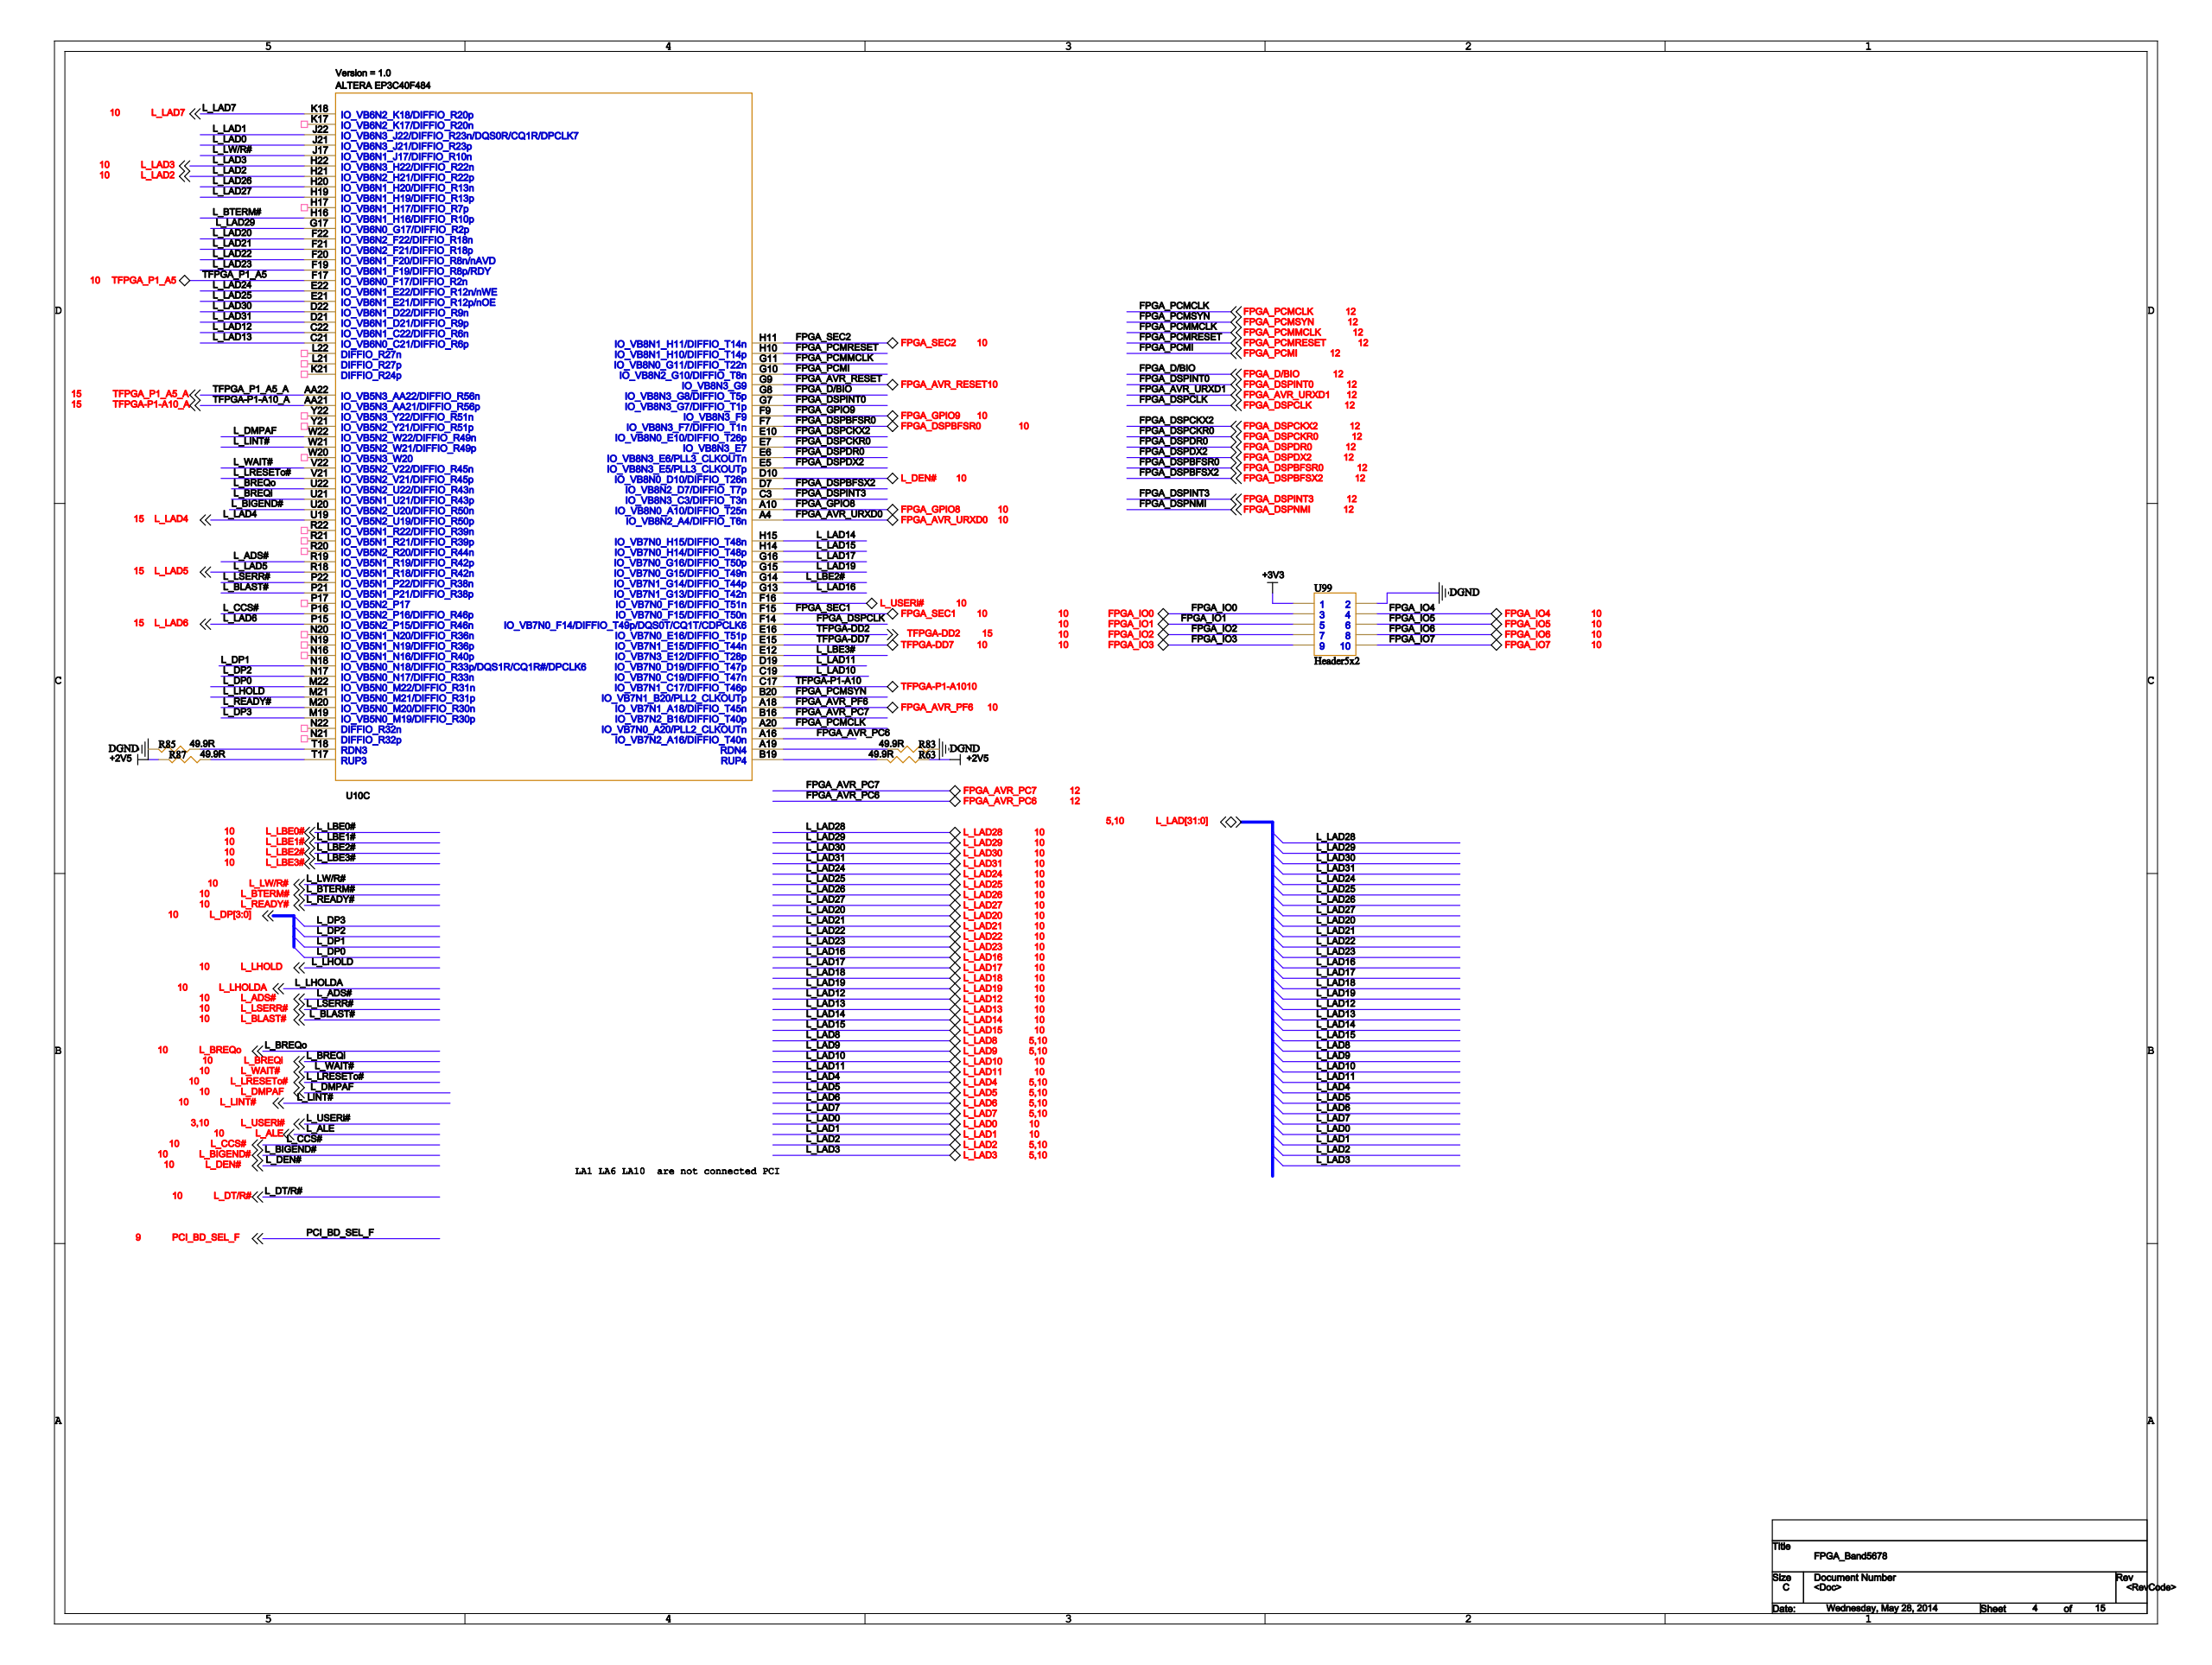Circuit board | Cadence Allegro | 669 parts | 806 nets | one sheet of the schematic
Parts on this sheet (reference | value | footprint):
R63 | 49.9R | R0603
R83 | 49.9R | R0603
R85 | 49.9R | R0603
R87 | 49.9R | R0603
U10 | EP3C40F484C8N | FBGA484
U99 | Header5x2 | ZIP10
Nets of these parts (net: part-pin ...):
DGND: R83-2 R85-2 U99-2
FPGA_SEC2: U10-H11
FPGA_SEC1: U10-F15
+3V3: U99-1
L_DP3: U10-M19
L_READY#: U10-M20
L_LHOLD: U10-M21
L_DP0: U10-M22
L_DP2: U10-N17
L_DP1: U10-N18
L_BLAST#: U10-P21
L_LSERR#: U10-P22
L_LAD5: U10-R18
L_ADS#: U10-R19
L_LAD6: U10-P15
L_CCS#: U10-P16
L_LAD4: U10-U19
L_BIGEND#: U10-U20
L_WAIT#: U10-V22
L_LINT#: U10-W21
L_DMPAF: U10-W22
TFPGA-P1-A10_A: U10-AA21
TFPGA_P1_A5_A: U10-AA22
L_LAD13: U10-C21
TFPGA_P1_A5: U10-F17
L_LAD29: U10-G17
L_LAD12: U10-C22
L_LAD31: U10-D21
L_LAD30: U10-D22
L_LAD25: U10-E21
L_LAD24: U10-E22
L_LAD23: U10-F19
L_LAD22: U10-F20
L_BTERM#: U10-H16
L_LAD27: U10-H19
L_LAD26: U10-H20
L_LW/R#: U10-J17
L_LAD21: U10-F21
L_LAD20: U10-F22
L_LAD2: U10-H21
L_LAD7: U10-K18
L_LAD3: U10-H22
L_LAD0: U10-J21
L_LAD1: U10-J22
FPGA_PCMCLK: U10-A20
L_LAD10: U10-C19
L_LAD11: U10-D19
TFPGA-DD2: U10-E16
FPGA_DSPCLK: U10-F14
L_LAD19: U10-G15
L_LAD17: U10-G16
L_LAD15: U10-H14
L_LAD14: U10-H15
FPGA_AVR_PF6: U10-A18
FPGA_PCMSYN: U10-B20
TFPGA-P1-A10: U10-C17
TFPGA-DD7: U10-E15
L_LAD16: U10-G13
L_LBE2#: U10-G14
FPGA_AVR_PC6: U10-A16
FPGA_AVR_PC7: U10-B16
L_LBE3#: U10-E12
FPGA_GPIO8: U10-A10
L_DEN#: U10-D10
FPGA_DSPCKX2: U10-E10
FPGA_PCMMCLK: U10-G11
FPGA_PCMRESET: U10-H10
FPGA_AVR_URXD0: U10-A4
FPGA_DSPBFSX2: U10-D7
FPGA_PCMI: U10-G10
FPGA_DSPINT3: U10-C3
FPGA_DSPDX2: U10-E5
FPGA_DSPDR0: U10-E6
FPGA_DSPCKR0: U10-E7
FPGA_DSPBFSR0: U10-F7
FPGA_GPIO9: U10-F9
FPGA_DSPINT0: U10-G7
FPGA_D/BIO: U10-G8
FPGA_AVR_RESET: U10-G9
N56702786: R85-1 U10-T18
N56697321: R83-1 U10-A19
N56702788: R87-1 U10-T17
N56697331: R63-1 U10-B19
FPGA_IO2: U99-7
FPGA_IO3: U99-9
FPGA_IO7: U99-10
FPGA_IO1: U99-5
FPGA_IO0: U99-3
FPGA_IO5: U99-6
FPGA_IO6: U99-8
FPGA_IO4: U99-4
+2V5: R63-2 R87-2